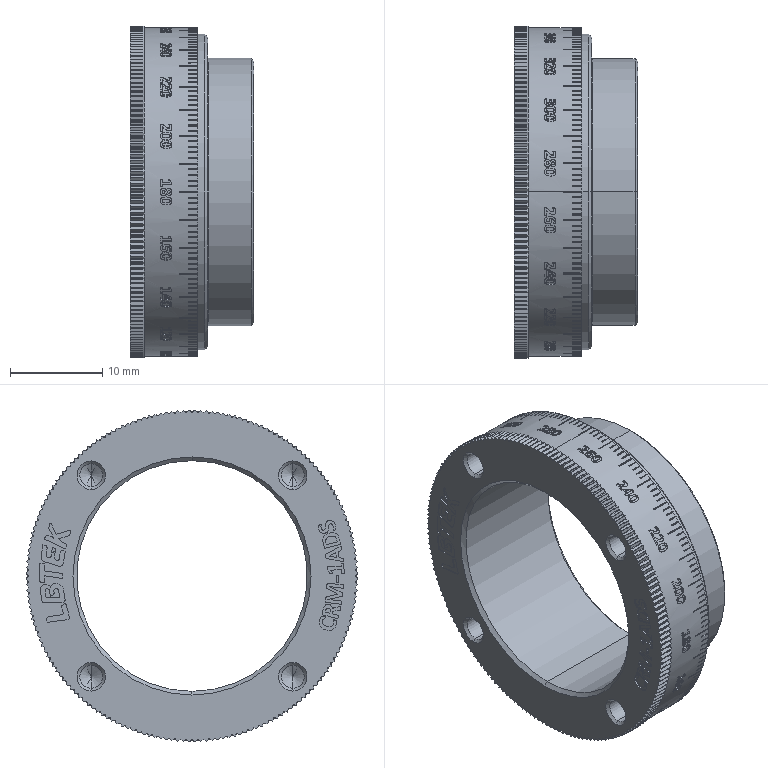Part | STEP file | 1 solid | 2943 faces | box 13.4 x 35.988 x 35.988 mm | volume 4856 mm3 | plane 1651 | cylinder 681 | spline 583 | cone 24 | torus 4 | commonest cylinder face diameters 0.12 x540 35.4 x48 35.6 x36 2.5 x8 0.176 x5 0.452 x5